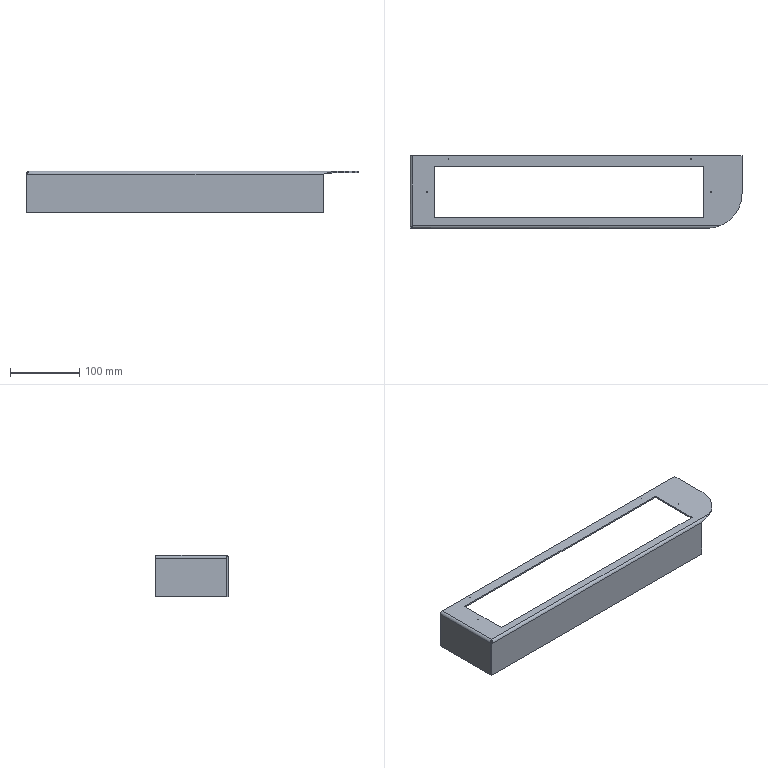Part | NX | features solid 2 | 1 solid | 40 faces | box 480 x 105 x 60 mm | volume 101636 mm3 | plane 23 | cylinder 13 | spline 4 | commonest cylinder face diameters 1 x8 4 x2 8 x2 100 x1